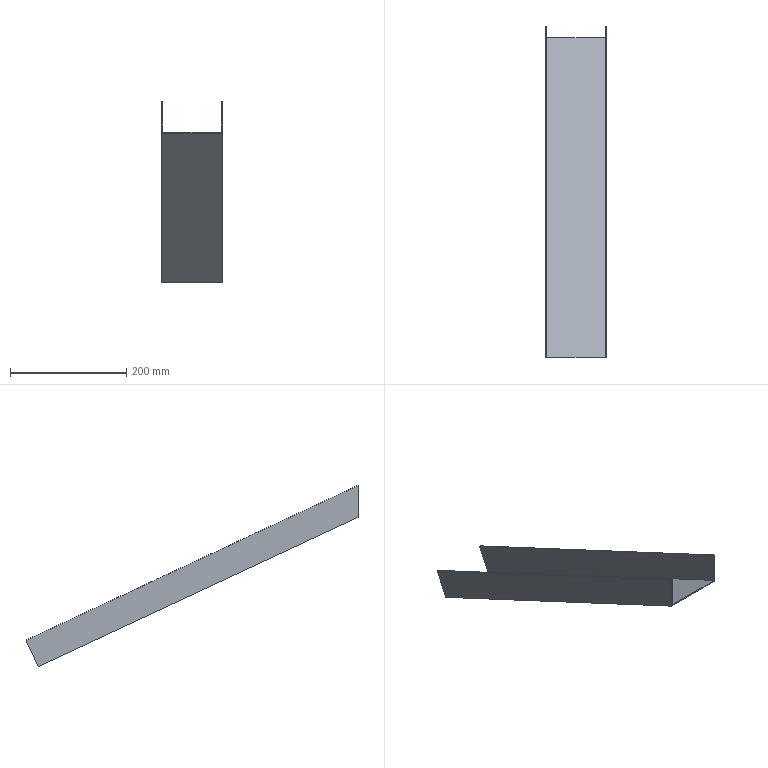Part | NX | features solid 2 | 1 solid | 10 faces | box 105 x 571.131 x 311.638 mm | volume 246383 mm3 | plane 10
STEP:
#1=CARTESIAN_POINT('',(160.,475.,-131.632));
#2=VERTEX_POINT('',#1);
#3=CARTESIAN_POINT('',(162.,475.,-131.632));
#4=VERTEX_POINT('',#3);
#5=CARTESIAN_POINT('',(-1360.,475.,-131.632));
#6=DIRECTION('',(1.,0.,0.));
#7=VECTOR('',#6,1000.);
#8=LINE('',#5,#7);
#9=EDGE_CURVE('',#2,#4,#8,.T.);
#10=ORIENTED_EDGE('',*,*,#9,.F.);
#11=CARTESIAN_POINT('',(160.,475.,-186.801));
#12=VERTEX_POINT('',#11);
#13=CARTESIAN_POINT('',(160.,475.,-215.));
#14=DIRECTION('',(0.,0.,-1.));
#15=VECTOR('',#14,1000.);
#16=LINE('',#13,#15);
#17=EDGE_CURVE('',#2,#12,#16,.T.);
#18=ORIENTED_EDGE('',*,*,#17,.T.);
#19=CARTESIAN_POINT('',(265.,475.,-186.801));
#20=VERTEX_POINT('',#19);
#21=CARTESIAN_POINT('',(-1360.,475.,-186.801));
#22=DIRECTION('',(1.,0.,0.));
#23=VECTOR('',#22,1000.);
#24=LINE('',#21,#23);
#25=EDGE_CURVE('',#12,#20,#24,.T.);
#26=ORIENTED_EDGE('',*,*,#25,.T.);
#27=CARTESIAN_POINT('',(265.,475.,-131.632));
#28=VERTEX_POINT('',#27);
#29=CARTESIAN_POINT('',(265.,475.,-175.106));
#30=DIRECTION('',(0.,0.,-1.));
#31=VECTOR('',#30,1000.);
#32=LINE('',#29,#31);
#33=EDGE_CURVE('',#28,#20,#32,.T.);
#34=ORIENTED_EDGE('',*,*,#33,.F.);
#35=CARTESIAN_POINT('',(263.,475.,-131.632));
#36=VERTEX_POINT('',#35);
#37=CARTESIAN_POINT('',(-1360.,475.,-131.632));
#38=DIRECTION('',(1.,0.,0.));
#39=VECTOR('',#38,1000.);
#40=LINE('',#37,#39);
#41=EDGE_CURVE('',#36,#28,#40,.T.);
#42=ORIENTED_EDGE('',*,*,#41,.F.);
#43=CARTESIAN_POINT('',(263.,475.,-184.594));
#44=VERTEX_POINT('',#43);
#45=CARTESIAN_POINT('',(263.,475.,-175.106));
#46=DIRECTION('',(0.,0.,-1.));
#47=VECTOR('',#46,1000.);
#48=LINE('',#45,#47);
#49=EDGE_CURVE('',#36,#44,#48,.T.);
#50=ORIENTED_EDGE('',*,*,#49,.T.);
#51=CARTESIAN_POINT('',(162.,475.,-184.594));
#52=VERTEX_POINT('',#51);
#53=CARTESIAN_POINT('',(-1360.,475.,-184.594));
#54=DIRECTION('',(1.,0.,0.));
#55=VECTOR('',#54,1000.);
#56=LINE('',#53,#55);
#57=EDGE_CURVE('',#52,#44,#56,.T.);
#58=ORIENTED_EDGE('',*,*,#57,.F.);
#59=CARTESIAN_POINT('',(162.,475.,-215.));
#60=DIRECTION('',(0.,0.,-1.));
#61=VECTOR('',#60,1000.);
#62=LINE('',#59,#61);
#63=EDGE_CURVE('',#4,#52,#62,.T.);
#64=ORIENTED_EDGE('',*,*,#63,.F.);
#65=EDGE_LOOP('',(#10,#18,#26,#34,#42,#50,#58,#64));
#66=FACE_BOUND('',#65,.T.);
#67=CARTESIAN_POINT('',(-1360.,475.,-215.));
#68=DIRECTION('',(0.,-1.,0.));
#69=DIRECTION('',(-1.,0.,0.));
#70=AXIS2_PLACEMENT_3D('',#67,#68,#69);
#71=PLANE('',#70);
#72=ADVANCED_FACE('',(#66),#71,.T.);
#73=CARTESIAN_POINT('',(265.,1046.131,-397.955));
#74=VERTEX_POINT('',#73);
#75=CARTESIAN_POINT('',(263.,1046.131,-397.955));
#76=VERTEX_POINT('',#75);
#77=CARTESIAN_POINT('',(160.,1046.131,-397.955));
#78=DIRECTION('',(-1.,0.,0.));
#79=VECTOR('',#78,1000.);
#80=LINE('',#77,#79);
#81=EDGE_CURVE('',#74,#76,#80,.T.);
#82=ORIENTED_EDGE('',*,*,#81,.F.);
#83=CARTESIAN_POINT('',(265.,1025.,-443.27));
#84=VERTEX_POINT('',#83);
#85=CARTESIAN_POINT('',(265.,1046.131,-397.955));
#86=DIRECTION('',(0.,-0.4226,-0.9063));
#87=VECTOR('',#86,1000.);
#88=LINE('',#85,#87);
#89=EDGE_CURVE('',#74,#84,#88,.T.);
#90=ORIENTED_EDGE('',*,*,#89,.T.);
#91=CARTESIAN_POINT('',(160.,1025.,-443.27));
#92=VERTEX_POINT('',#91);
#93=CARTESIAN_POINT('',(160.,1025.,-443.27));
#94=DIRECTION('',(-1.,0.,0.));
#95=VECTOR('',#94,1000.);
#96=LINE('',#93,#95);
#97=EDGE_CURVE('',#84,#92,#96,.T.);
#98=ORIENTED_EDGE('',*,*,#97,.T.);
#99=CARTESIAN_POINT('',(160.,1046.131,-397.955));
#100=VERTEX_POINT('',#99);
#101=CARTESIAN_POINT('',(160.,1046.131,-397.955));
#102=DIRECTION('',(0.,-0.4226,-0.9063));
#103=VECTOR('',#102,1000.);
#104=LINE('',#101,#103);
#105=EDGE_CURVE('',#100,#92,#104,.T.);
#106=ORIENTED_EDGE('',*,*,#105,.F.);
#107=CARTESIAN_POINT('',(162.,1046.131,-397.955));
#108=VERTEX_POINT('',#107);
#109=CARTESIAN_POINT('',(160.,1046.131,-397.955));
#110=DIRECTION('',(-1.,0.,0.));
#111=VECTOR('',#110,1000.);
#112=LINE('',#109,#111);
#113=EDGE_CURVE('',#108,#100,#112,.T.);
#114=ORIENTED_EDGE('',*,*,#113,.F.);
#115=CARTESIAN_POINT('',(162.,1025.845,-441.458));
#116=VERTEX_POINT('',#115);
#117=CARTESIAN_POINT('',(162.,1046.131,-397.955));
#118=DIRECTION('',(0.,-0.4226,-0.9063));
#119=VECTOR('',#118,1000.);
#120=LINE('',#117,#119);
#121=EDGE_CURVE('',#108,#116,#120,.T.);
#122=ORIENTED_EDGE('',*,*,#121,.T.);
#123=CARTESIAN_POINT('',(263.,1025.845,-441.458));
#124=VERTEX_POINT('',#123);
#125=CARTESIAN_POINT('',(160.,1025.845,-441.458));
#126=DIRECTION('',(-1.,0.,0.));
#127=VECTOR('',#126,1000.);
#128=LINE('',#125,#127);
#129=EDGE_CURVE('',#124,#116,#128,.T.);
#130=ORIENTED_EDGE('',*,*,#129,.F.);
#131=CARTESIAN_POINT('',(263.,1046.131,-397.955));
#132=DIRECTION('',(0.,-0.4226,-0.9063));
#133=VECTOR('',#132,1000.);
#134=LINE('',#131,#133);
#135=EDGE_CURVE('',#76,#124,#134,.T.);
#136=ORIENTED_EDGE('',*,*,#135,.F.);
#137=EDGE_LOOP('',(#82,#90,#98,#106,#114,#122,#130,#136));
#138=FACE_BOUND('',#137,.T.);
#139=CARTESIAN_POINT('',(160.,1046.131,-397.955));
#140=DIRECTION('',(0.,0.9063,-0.4226));
#141=DIRECTION('',(0.,-0.4226,-0.9063));
#142=AXIS2_PLACEMENT_3D('',#139,#140,#141);
#143=PLANE('',#142);
#144=ADVANCED_FACE('',(#138),#143,.T.);
#145=ORIENTED_EDGE('',*,*,#113,.T.);
#146=CARTESIAN_POINT('',(160.,568.231,-175.106));
#147=DIRECTION('',(0.,-0.9063,0.4226));
#148=VECTOR('',#147,1000.);
#149=LINE('',#146,#148);
#150=EDGE_CURVE('',#100,#2,#149,.T.);
#151=ORIENTED_EDGE('',*,*,#150,.T.);
#152=ORIENTED_EDGE('',*,*,#9,.T.);
#153=CARTESIAN_POINT('',(162.,568.231,-175.106));
#154=DIRECTION('',(0.,-0.9063,0.4226));
#155=VECTOR('',#154,1000.);
#156=LINE('',#153,#155);
#157=EDGE_CURVE('',#108,#4,#156,.T.);
#158=ORIENTED_EDGE('',*,*,#157,.F.);
#159=EDGE_LOOP('',(#145,#151,#152,#158));
#160=FACE_BOUND('',#159,.T.);
#161=CARTESIAN_POINT('',(160.,568.231,-175.106));
#162=DIRECTION('',(0.,-0.4226,-0.9063));
#163=DIRECTION('',(-1.,0.,0.));
#164=AXIS2_PLACEMENT_3D('',#161,#162,#163);
#165=PLANE('',#164);
#166=ADVANCED_FACE('',(#160),#165,.F.);
#167=CARTESIAN_POINT('',(160.,547.1,-220.422));
#168=DIRECTION('',(0.,-0.9063,0.4226));
#169=VECTOR('',#168,1000.);
#170=LINE('',#167,#169);
#171=EDGE_CURVE('',#92,#12,#170,.T.);
#172=ORIENTED_EDGE('',*,*,#171,.T.);
#173=ORIENTED_EDGE('',*,*,#17,.F.);
#174=ORIENTED_EDGE('',*,*,#150,.F.);
#175=ORIENTED_EDGE('',*,*,#105,.T.);
#176=EDGE_LOOP('',(#172,#173,#174,#175));
#177=FACE_BOUND('',#176,.T.);
#178=CARTESIAN_POINT('',(160.,568.231,-175.106));
#179=DIRECTION('',(-1.,0.,0.));
#180=DIRECTION('',(0.,0.,1.));
#181=AXIS2_PLACEMENT_3D('',#178,#179,#180);
#182=PLANE('',#181);
#183=ADVANCED_FACE('',(#177),#182,.T.);
#184=CARTESIAN_POINT('',(265.,547.1,-220.422));
#185=DIRECTION('',(0.,0.9063,-0.4226));
#186=VECTOR('',#185,1000.);
#187=LINE('',#184,#186);
#188=EDGE_CURVE('',#20,#84,#187,.T.);
#189=ORIENTED_EDGE('',*,*,#188,.T.);
#190=ORIENTED_EDGE('',*,*,#89,.F.);
#191=CARTESIAN_POINT('',(265.,568.231,-175.106));
#192=DIRECTION('',(0.,0.9063,-0.4226));
#193=VECTOR('',#192,1000.);
#194=LINE('',#191,#193);
#195=EDGE_CURVE('',#28,#74,#194,.T.);
#196=ORIENTED_EDGE('',*,*,#195,.F.);
#197=ORIENTED_EDGE('',*,*,#33,.T.);
#198=EDGE_LOOP('',(#189,#190,#196,#197));
#199=FACE_BOUND('',#198,.T.);
#200=CARTESIAN_POINT('',(265.,568.231,-175.106));
#201=DIRECTION('',(1.,0.,0.));
#202=DIRECTION('',(0.,0.,-1.));
#203=AXIS2_PLACEMENT_3D('',#200,#201,#202);
#204=PLANE('',#203);
#205=ADVANCED_FACE('',(#199),#204,.T.);
#206=ORIENTED_EDGE('',*,*,#41,.T.);
#207=ORIENTED_EDGE('',*,*,#195,.T.);
#208=ORIENTED_EDGE('',*,*,#81,.T.);
#209=CARTESIAN_POINT('',(263.,568.231,-175.106));
#210=DIRECTION('',(0.,0.9063,-0.4226));
#211=VECTOR('',#210,1000.);
#212=LINE('',#209,#211);
#213=EDGE_CURVE('',#36,#76,#212,.T.);
#214=ORIENTED_EDGE('',*,*,#213,.F.);
#215=EDGE_LOOP('',(#206,#207,#208,#214));
#216=FACE_BOUND('',#215,.T.);
#217=CARTESIAN_POINT('',(160.,568.231,-175.106));
#218=DIRECTION('',(0.,-0.4226,-0.9063));
#219=DIRECTION('',(-1.,0.,0.));
#220=AXIS2_PLACEMENT_3D('',#217,#218,#219);
#221=PLANE('',#220);
#222=ADVANCED_FACE('',(#216),#221,.F.);
#223=ORIENTED_EDGE('',*,*,#171,.F.);
#224=ORIENTED_EDGE('',*,*,#97,.F.);
#225=ORIENTED_EDGE('',*,*,#188,.F.);
#226=ORIENTED_EDGE('',*,*,#25,.F.);
#227=EDGE_LOOP('',(#223,#224,#225,#226));
#228=FACE_BOUND('',#227,.T.);
#229=CARTESIAN_POINT('',(160.,547.1,-220.422));
#230=DIRECTION('',(0.,-0.4226,-0.9063));
#231=DIRECTION('',(-1.,0.,0.));
#232=AXIS2_PLACEMENT_3D('',#229,#230,#231);
#233=PLANE('',#232);
#234=ADVANCED_FACE('',(#228),#233,.T.);
#235=CARTESIAN_POINT('',(162.,547.945,-218.609));
#236=DIRECTION('',(0.,-0.9063,0.4226));
#237=VECTOR('',#236,1000.);
#238=LINE('',#235,#237);
#239=EDGE_CURVE('',#116,#52,#238,.T.);
#240=ORIENTED_EDGE('',*,*,#239,.F.);
#241=ORIENTED_EDGE('',*,*,#121,.F.);
#242=ORIENTED_EDGE('',*,*,#157,.T.);
#243=ORIENTED_EDGE('',*,*,#63,.T.);
#244=EDGE_LOOP('',(#240,#241,#242,#243));
#245=FACE_BOUND('',#244,.T.);
#246=CARTESIAN_POINT('',(162.,568.231,-175.106));
#247=DIRECTION('',(-1.,0.,0.));
#248=DIRECTION('',(0.,0.,1.));
#249=AXIS2_PLACEMENT_3D('',#246,#247,#248);
#250=PLANE('',#249);
#251=ADVANCED_FACE('',(#245),#250,.F.);
#252=CARTESIAN_POINT('',(263.,547.945,-218.609));
#253=DIRECTION('',(0.,0.9063,-0.4226));
#254=VECTOR('',#253,1000.);
#255=LINE('',#252,#254);
#256=EDGE_CURVE('',#44,#124,#255,.T.);
#257=ORIENTED_EDGE('',*,*,#256,.F.);
#258=ORIENTED_EDGE('',*,*,#49,.F.);
#259=ORIENTED_EDGE('',*,*,#213,.T.);
#260=ORIENTED_EDGE('',*,*,#135,.T.);
#261=EDGE_LOOP('',(#257,#258,#259,#260));
#262=FACE_BOUND('',#261,.T.);
#263=CARTESIAN_POINT('',(263.,568.231,-175.106));
#264=DIRECTION('',(1.,0.,0.));
#265=DIRECTION('',(0.,0.,-1.));
#266=AXIS2_PLACEMENT_3D('',#263,#264,#265);
#267=PLANE('',#266);
#268=ADVANCED_FACE('',(#262),#267,.F.);
#269=ORIENTED_EDGE('',*,*,#239,.T.);
#270=ORIENTED_EDGE('',*,*,#57,.T.);
#271=ORIENTED_EDGE('',*,*,#256,.T.);
#272=ORIENTED_EDGE('',*,*,#129,.T.);
#273=EDGE_LOOP('',(#269,#270,#271,#272));
#274=FACE_BOUND('',#273,.T.);
#275=CARTESIAN_POINT('',(160.,547.945,-218.609));
#276=DIRECTION('',(0.,-0.4226,-0.9063));
#277=DIRECTION('',(-1.,0.,0.));
#278=AXIS2_PLACEMENT_3D('',#275,#276,#277);
#279=PLANE('',#278);
#280=ADVANCED_FACE('',(#274),#279,.F.);
#281=CLOSED_SHELL('',(#72,#144,#166,#183,#205,#222,#234,#251,#268,#280));
#282=MANIFOLD_SOLID_BREP('',#281);
#283=(LENGTH_UNIT()NAMED_UNIT(*)SI_UNIT(.MILLI.,.METRE.));
#284=UNCERTAINTY_MEASURE_WITH_UNIT(LENGTH_MEASURE(0.00001),#283,'','');
#285=(NAMED_UNIT(*)PLANE_ANGLE_UNIT()SI_UNIT($,.RADIAN.));
#286=(NAMED_UNIT(*)SI_UNIT($,.STERADIAN.)SOLID_ANGLE_UNIT());
#287=(GEOMETRIC_REPRESENTATION_CONTEXT(3)GLOBAL_UNCERTAINTY_ASSIGNED_CONTEXT((#284))GLOBAL_UNIT_ASSIGNED_CONTEXT((#283,#285,#286))REPRESENTATION_CONTEXT('',''));
#288=ADVANCED_BREP_SHAPE_REPRESENTATION('',(#282),#287);